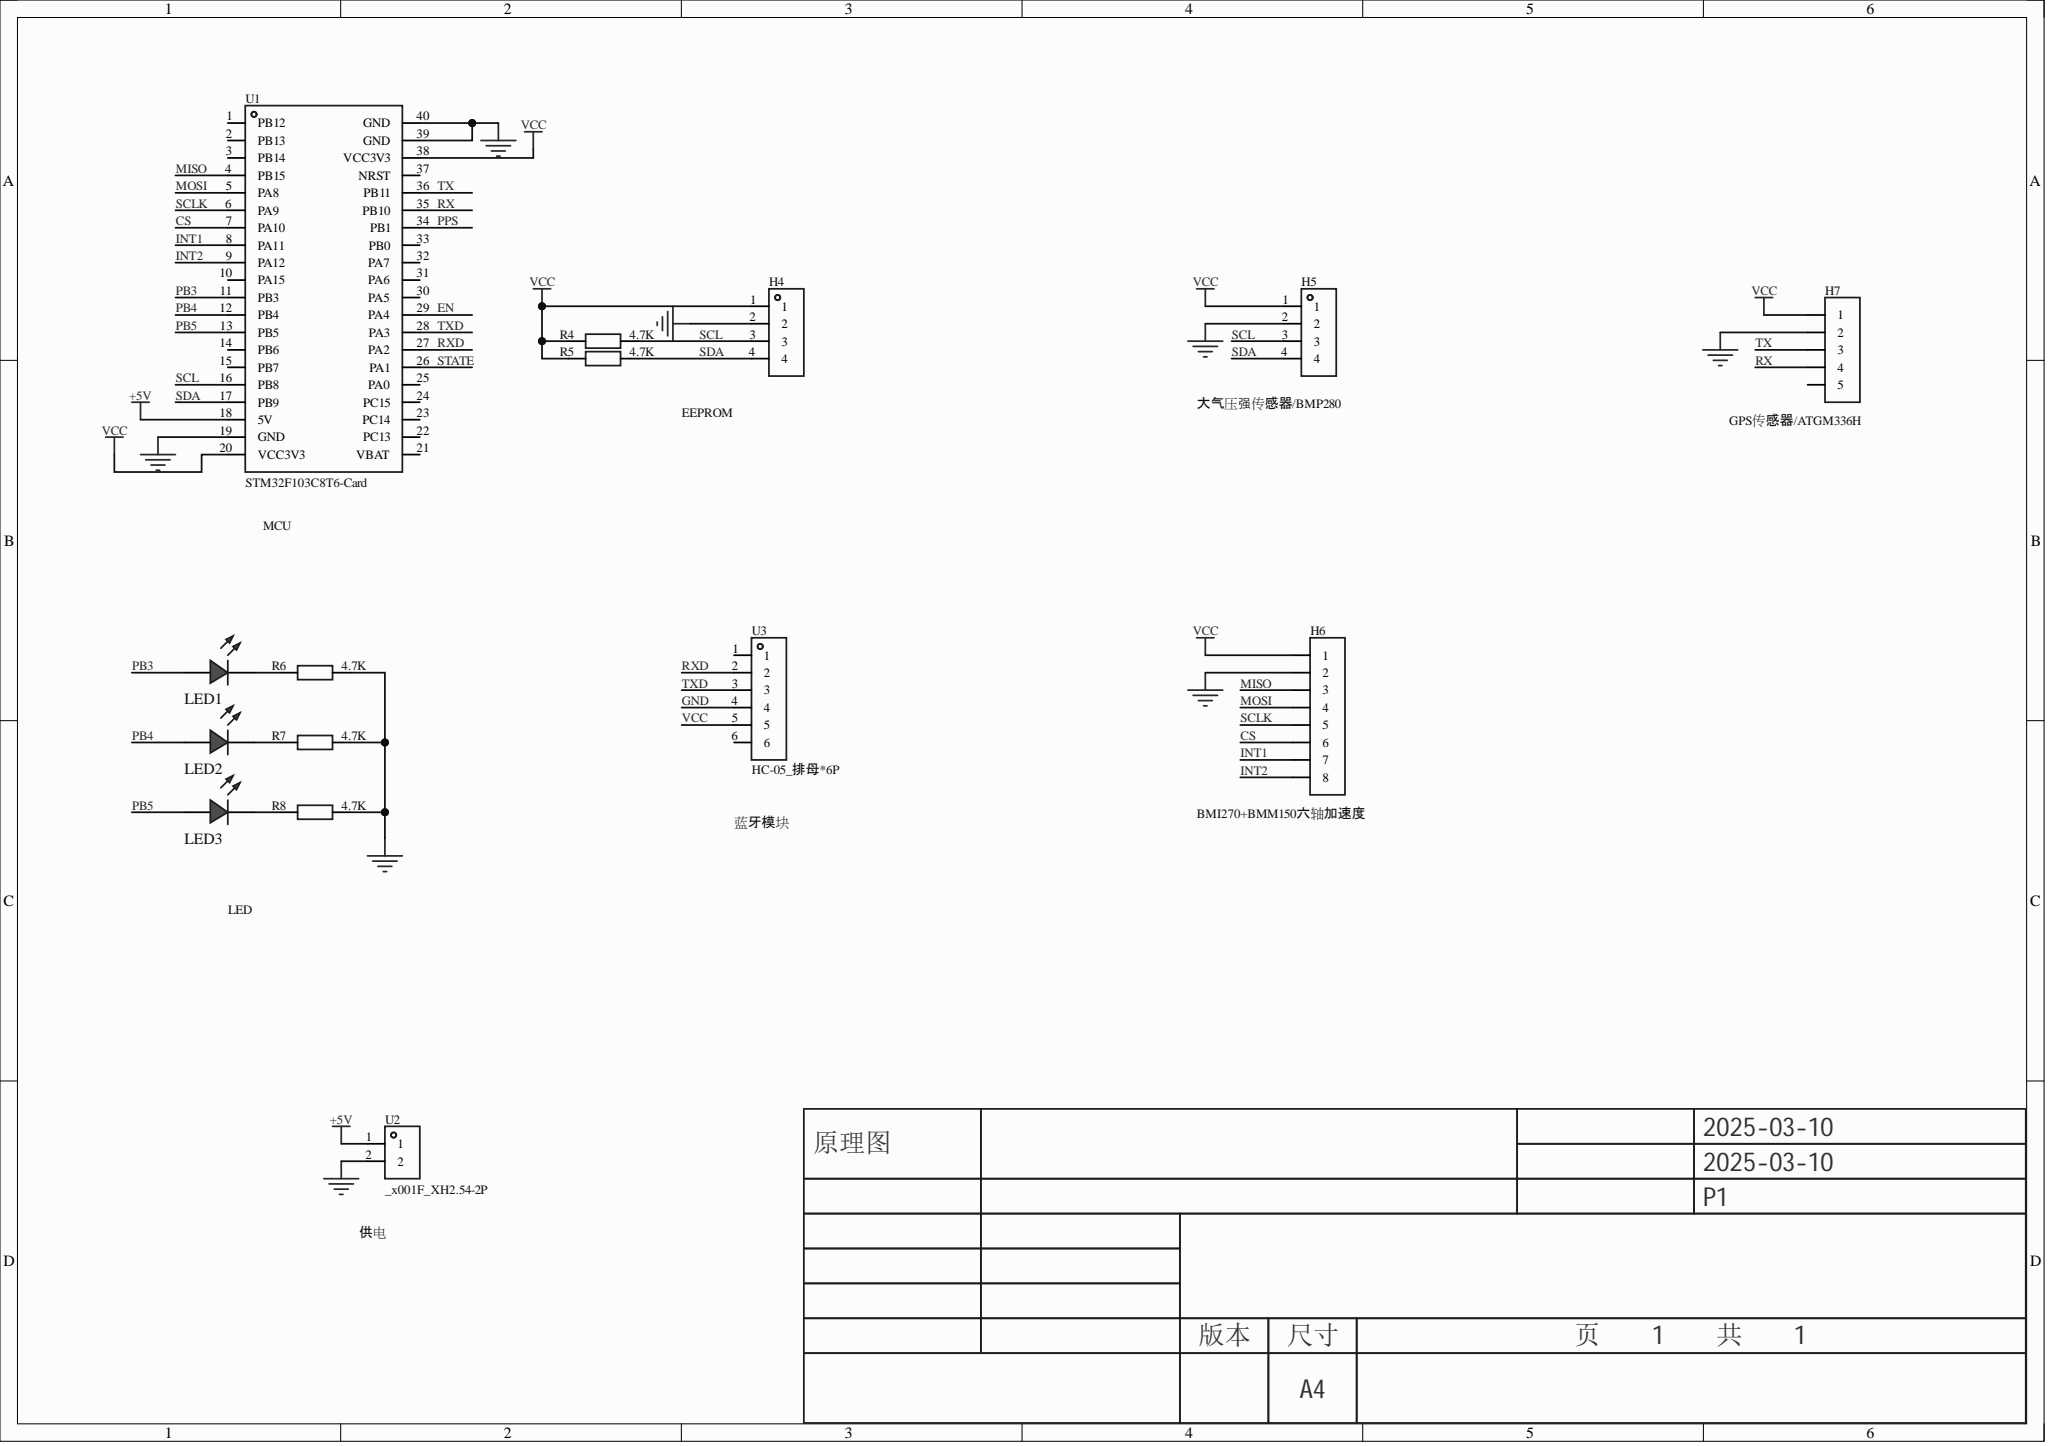Circuit board | Altium Designer | 15 parts | 21 nets
Bill of materials:
Comment,Description,Designator,Footprint,LibRef,Quantity
"","","H4, H5","HDR-TH_4P-P2.54-V-F","HDR-F_2.54_1x4P","2"
"","","H6","HDR-TH_8P-P2.54-V-F-1","HDR-F_2.54_1x8P","1"
"","","H7","HDR-TH_5P-P2.54-V-F","HDR-F_2.54_1x5P","1"
"","","LED1, LED2, LED3","LED_0805","LED_0805-R","3"
"4.7K","","R4, R5, R6, R7, R8","R0805","Res_0805","5"
"STM32F103C8T6-Card","","U1","CONN-TH_L53.3-W22.9_STM32F103C8T6-CARD","STM32F103C8T6-Card","1"
"_x001F_XH2.54-2P","","U2","CONN-TH_2P-P2.54-V","_x001F_XH2.54-2P","1"
"HC-05_排母*6P","","U3","HDR-TH_6P-P2.50-V-F-R1-C6","HC-05_排母*6P","1"
Netlist (Protel format):
[
H4
HDR-TH_4P-P2.54-V-F




]
[
H5
HDR-TH_4P-P2.54-V-F




]
[
H6
HDR-TH_8P-P2.54-V-F-1




]
[
H7
HDR-TH_5P-P2.54-V-F




]
[
LED1
LED_0805




]
[
LED2
LED_0805




]
[
LED3
LED_0805




]
[
R4
R0805
4.7K



]
[
R5
R0805
4.7K



]
[
R6
R0805
4.7K



]
[
R7
R0805
4.7K



]
[
R8
R0805
4.7K



]
[
U1
CONN-TH_L53.3-W22.9_STM32F103C8T6-CARD
STM32F103C8T6-Card



]
[
U2
CONN-TH_2P-P2.54-V
_x001F_XH2.54-2P



]
[
U3
HDR-TH_6P-P2.50-V-F-R1-C6
HC-05_排母*6P



]
(
VCC
H4-1
H5-1
H6-1
H7-1
R4-1
R5-1
U1-20
U1-38
U3-5
)
(
TXD
U1-28
U3-3
)
(
TX
H7-3
U1-36
)
(
SDA
H4-4
H5-4
R5-2
U1-17
)
(
SCLK
H6-5
U1-6
)
(
SCL
H4-3
H5-3
R4-2
U1-16
)
(
RXD
U1-27
U3-2
)
(
RX
H7-4
U1-35
)
(
PB5
LED3-2
U1-13
)
(
PB4
LED2-2
U1-12
)
(
PB3
LED1-2
U1-11
)
(
NetLED3_1
LED3-1
R8-1
)
(
NetLED2_1
LED2-1
R7-1
)
(
NetLED1_1
LED1-1
R6-1
)
(
MOSI
H6-4
U1-5
)
(
MISO
H6-3
U1-4
)
(
INT2
H6-8
U1-9
)
(
INT1
H6-7
U1-8
)
(
GND
H4-2
H5-2
H6-2
H7-2
R6-2
R7-2
R8-2
U1-19
U1-39
U1-40
U2-2
U3-4
)
(
CS
H6-6
U1-7
)
(
+5V
U1-18
U2-1
)